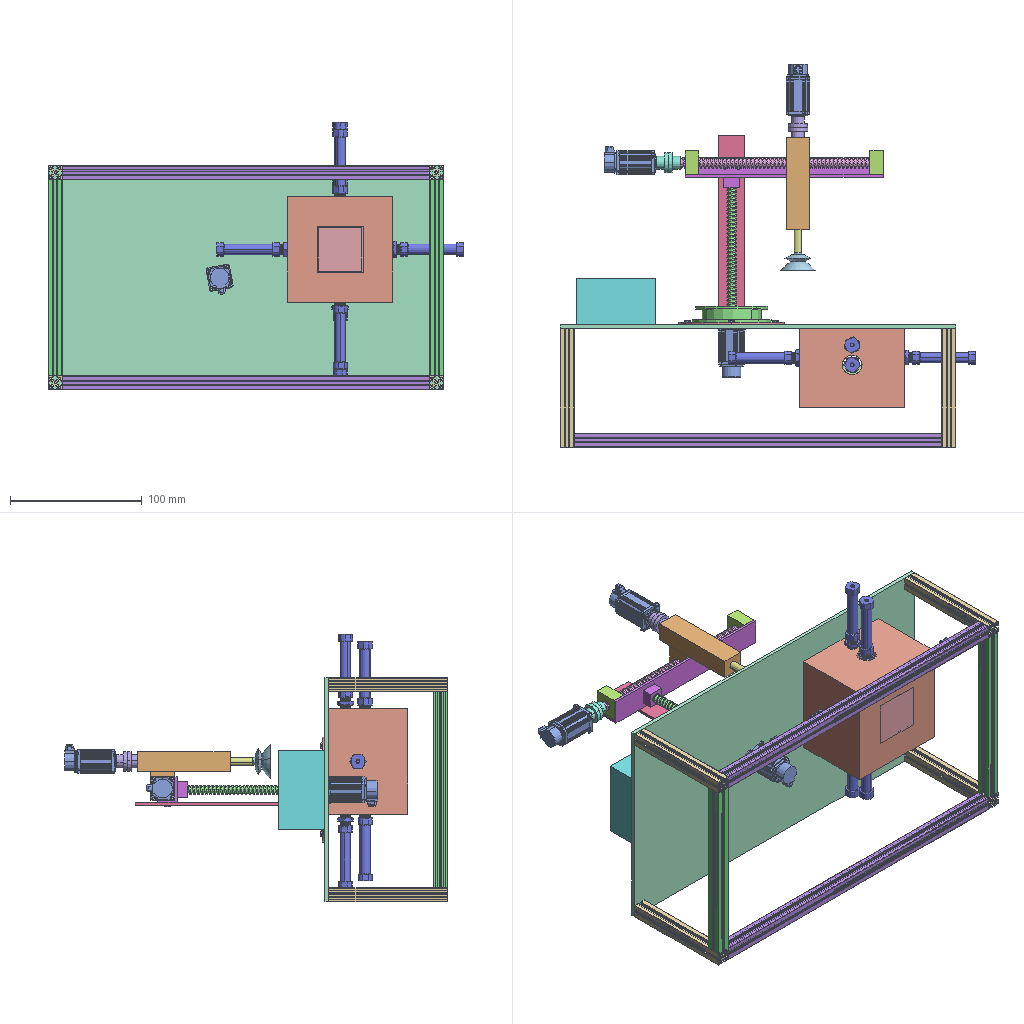Assembly | SolidWorks | 16 different items | 29 placed | box 315 x 291 x 203 mm
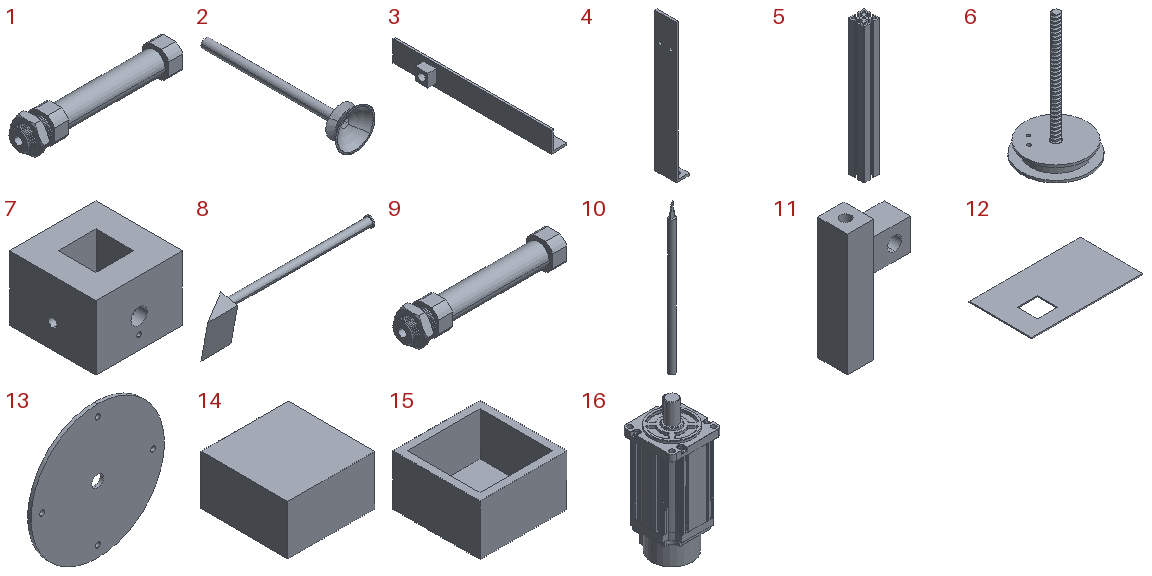Parts list (item | name | quantity | parent item | size | volume | features):
1 | (subassembly) | x2 | - | 56.5 x 12.702 x 11 mm | 2893 mm3 | -
2 | (subassembly) | x1 | - | 26 x 99 x 25.974 mm | 3520 mm3 | -
3 | - | x1 | - | 23 x 150 x 20 mm | 10744 mm3 | features ICE 2, Cut 1, Extrusion 1
4 | - | x1 | - | 12 x 20 x 130 mm | 5543 mm3 | features Cut 2, Extrusion 1, ICE 1
5 | - | x4 | - | 10.5 x 10.5 x 90 mm | 4956 mm3 | features ICE 3, Extrusion 1, Scale 1
6 | - | x1 | - | 60 x 60 x 110.002 mm | 25433 mm3 | features ICE 3, Cut 2, Extrusion 1, Helix 1, SweepCut 1
7 | - | x1 | - | 80 x 80 x 60 mm | 271765 mm3 | features Cut 6, ICE 3, Extrusion 1
8 | - | x2 | in 1 | 73.75 x 10.739 x 16.01 mm | 1055 mm3 | features ICE 4, Cut 1, Helix 1, Revolution 1, Scale 1, SweepCut 1
9 | - | x6 | in 1 | 56.5 x 12.702 x 11 mm | 2893 mm3 | features ICE 3, Helix 2, SweepCut 2, Chamfer 1, RevCut 1, Revolution 1, Scale 1
10 | - | x2 | - | 3 x 3 x 73.338 mm | 473.804 mm3 | features ICE 2, Extrusion 1
11 | - | x1 | - | 37 x 17 x 70 mm | 21057 mm3 | features Cut 2, Extrusion 1, ICE 1
12 | - | x1 | - | 300 x 170 x 3 mm | 143925 mm3 | features Cut 1, Extrusion 1
13 | - | x1 | - | 80 x 2 x 80 mm | 9920 mm3 | features Cut 2, Extrusion 1
14 | - | x1 | - | 35 x 35 x 20 mm | 3809 mm3 | features Extrusion 1, Shell 1
15 | - | x1 | - | 60 x 60 x 35 mm | 51000 mm3 | features Extrusion 1, Shell 1
16 | - | x3 | - | 18 x 21.6 x 47.1 mm | 10038 mm3 | features BaseBody 1, Scale 1
Mates (type | each side: item.copy, entity, surface, feature):
Coincident | 13.1 face plane Boss-Extrude1 | 16.1 face plane Input 1
Parallel | 11.1 face plane Boss-Extrude2 | 16.2 face plane Input 1
Concentric | 13.1 face cylinder Cut-Extrude3 | 6.1 face cylinder Boss-Extrude2
Coincident | 13.1 face plane Boss-Extrude1 | 6.1 face plane Boss-Extrude1
Concentric | 6.1 face cylinder Cut-Extrude2 | 4.1 face cylinder Cut-Extrude1 | 2 times
Coincident | 6.1 face plane Boss-Extrude3 | 4.1 face plane Boss-Extrude1
Coincident | 6.1 face plane Boss-Extrude4 | 3.1 face plane Boss-Extrude1
Concentric | 6.1 face cylinder Boss-Extrude4 | 3.1 face cylinder Boss-Extrude4
Coincident | 4.1 face plane Boss-Extrude1 | 3.1 face plane Boss-Extrude1
Coincident | 11.1 face plane Boss-Extrude1 | 3.1 face plane Cut-Extrude1 | 2 times
InPlace | 13.1 face plane Boss-Extrude1 | 12.1 plane
InPlace | 12.1 face plane Boss-Extrude1 | 7.1 plane
Concentric | 7.1 face cylinder Boss-Extrude2 | 9.1 face cylinder Revolve1
Concentric | 7.1 face cylinder Boss-Extrude3 | 9.2 face cylinder Revolve1
Coincident | 7.1 face plane Boss-Extrude1 | 9.1 face plane Boss-Extrude3
Parallel | 7.1 face plane Cut-Extrude2 | 8.1 face
Concentric | 9.1 face cylinder Revolve1 | 8.2 face cylinder Revolve1
Parallel | 7.1 face plane Cut-Extrude3 | 8.2 face plane Boss-Extrude3
Coincident | 7.1 face plane Cut-Extrude3 | 8.3 face plane Boss-Extrude3
Concentric | 9.2 face cylinder Revolve1 | 8.3 face cylinder Revolve1
Coincident | 7.1 face plane Boss-Extrude1 | 9.2 face plane Boss-Extrude3
Concentric | 7.1 face cylinder Cut-Extrude6 | 9.3 face cylinder Revolve1
Coincident | 7.1 face plane Boss-Extrude1 | 9.3 face plane Boss-Extrude3
Concentric | 7.1 face cylinder Cut-Extrude6 | 9.4 face cylinder Revolve1
Coincident | 7.1 face plane Boss-Extrude1 | 9.4 face plane Boss-Extrude3
Concentric | 9.4 face cylinder Revolve1 | 10.1 face cylinder Boss-Extrude1
Parallel | 7.1 face plane Cut-Extrude2 | 10.1 face plane Boss-Extrude3
Concentric | 9.3 face cylinder Revolve1 | 10.2 face cylinder Boss-Extrude1
Parallel | 7.1 face plane Cut-Extrude2 | 10.2 face plane Boss-Extrude3
InPlace | 12.1 face plane Boss-Extrude1 | 15.1 plane
Coincident | 12.1 face plane Boss-Extrude1 | 5.1 face plane Boss-Extrude3 | 3 times
Coincident | 12.1 face plane Boss-Extrude1 | 5.2 face plane Boss-Extrude3 | 3 times
InPlace | 7.1 face plane Boss-Extrude1 | 14.1 plane
Concentric | 7.1 face cylinder Cut-Extrude8 | 9.5 face cylinder Revolve1
Coincident | 7.1 face plane Boss-Extrude1 | 9.5 face plane Revolve1
Concentric | 7.1 face cylinder Cut-Extrude8 | 9.6 face cylinder Revolve1
Coincident | 7.1 face plane Boss-Extrude1 | 9.6 face plane Revolve1